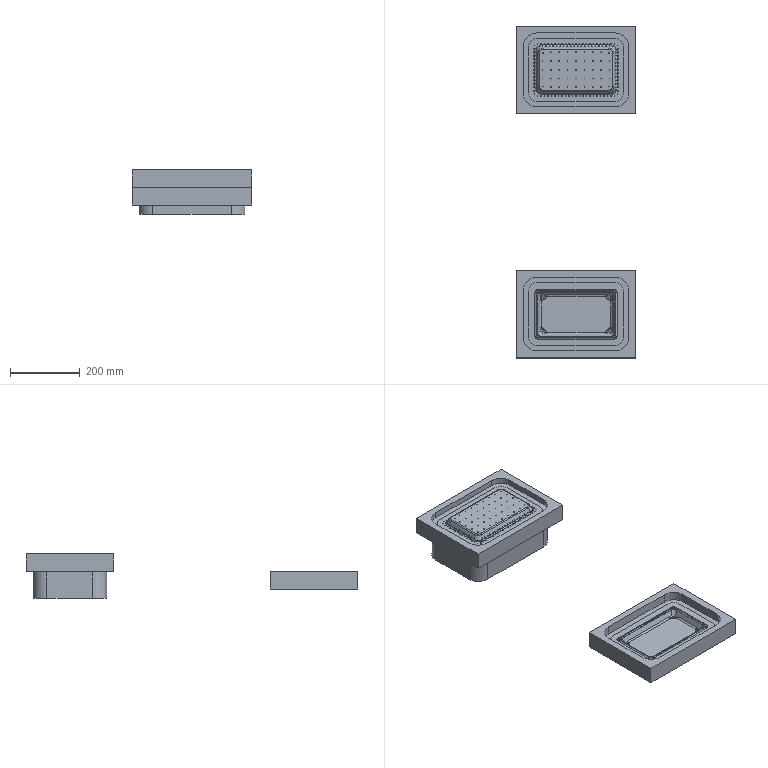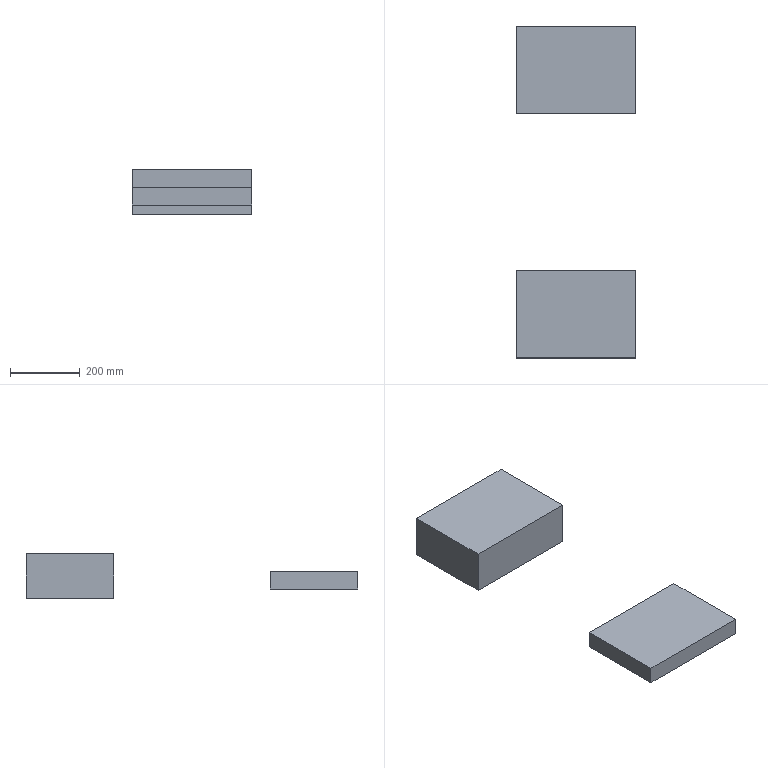CAM job | NX | 3-axis milling, drilling | part box 343.99 x 952.259 x 127.368 mm | stock box 343.99 x 952.259 x 127.368 mm
Tools:
number,name,description,diameter,corner_radius,flute_length,length,flutes
0,V2.0,Drilling Tool,2.0,0.0,35.0,50.0,2
0,D10,No Description,10.0,0.0,20.0,60.0,2
0,D4,No Description,4.0,0.0,0.0,20.0,2
0,D16R0.8,No Description,16.0,0.8,50.0,90.0,2
0,R2,No Description,4.0,2.0,0.0,20.0,2
Operations:
program,operation,operation_type,tool,method,geometry_group,spindle_rpm,surface_speed,feed_per_tooth,feed_cut,feed_plunge,cut_length_mm,path_length_mm,cut_time_min,machine_time_min
D-01,CAVITY_MILL_3,CavityMilling,D16R0.8,METHOD,24D,8000.0,402.0,0.25,4000.0,100.0,157661.907,159697.785,39.416,39.619
E-01,CAVITY_MILL_4,CavityMilling,D16R0.8,METHOD,24D_COPY,8000.0,402.0,0.25,4000.0,100.0,475202.366,485441.349,118.801,119.825
E-02,CAVITY_MILL_4_COPY,CavityMilling,D4,METHOD,24D_COPY,8000.0,402.0,0.25,4000.0,100.0,11868.533,13587.412,2.967,3.139
E-03,FACE_MILLING_3,FaceMilling,D10,METHOD,24D_COPY,8000.0,251.0,0.25,4000.0,100.0,4266.16,4613.425,1.067,1.101
E-04,CONTOUR_AREA_3,SurfaceContour,R2,METHOD,24D_COPY,9000.0,113.0,0.2222,4000.0,100.0,147474.941,147834.841,36.869,36.905
E-05,DRILLING,Operation,V2.0,METHOD,24D_COPY,2000.0,75.0,0.0375,150.0,0.0,950.0,5378.86,6.333,6.776
E-06,PLANAR_MILL_1,PlanarMilling,D10,METHOD,24D_COPY,8000.0,251.0,0.125,2000.0,100.0,17707.212,18063.277,8.854,8.889